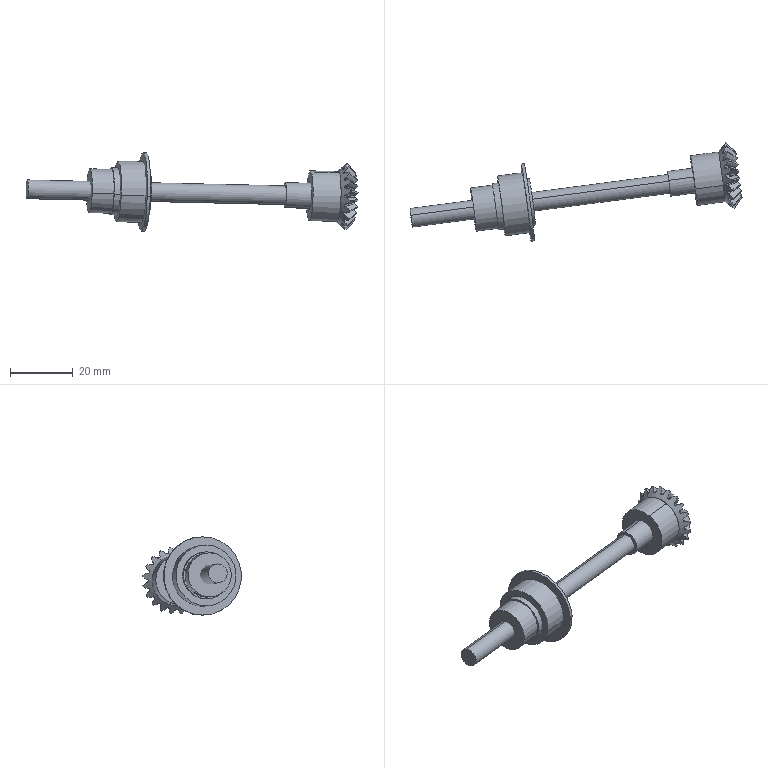Part | SolidWorks | 4 solids | 167 faces | box 105.964 x 31.504 x 25.016 mm | volume 9209 mm3 | spline 100 | cone 28 | cylinder 26 | plane 13 | commonest cylinder face diameters 8 x4 11.8 x4 15 x4 3 x2 5 x2 6 x2